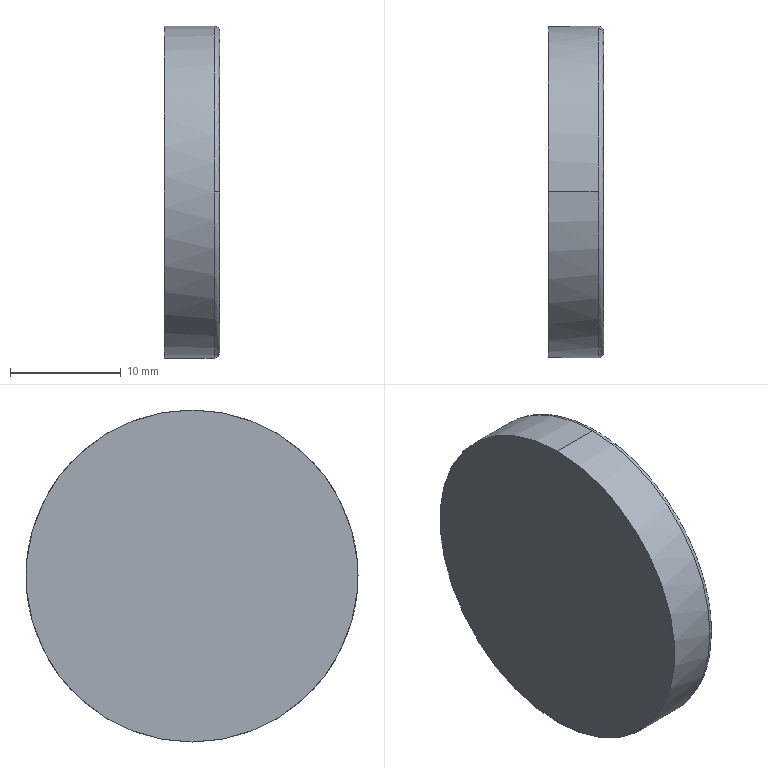Part | STEP file | ESG1 | 1 solid | 6 faces | box 5 x 30 x 30 mm | volume 3530 mm3 | spline 2 | cylinder 2 | plane 2 | commonest cylinder face diameters 30 x2